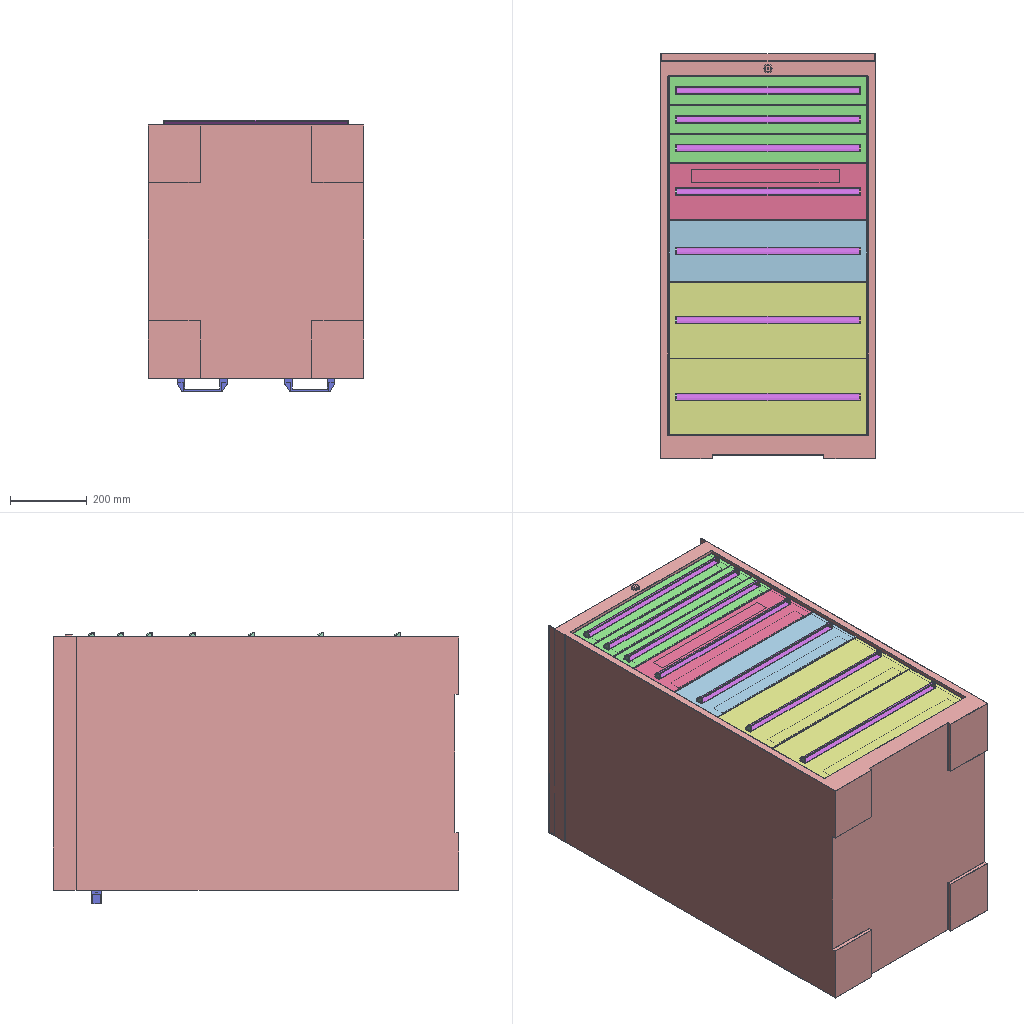Assembly | SolidWorks | 19 different items | 71 placed | box 560 x 1055 x 707 mm
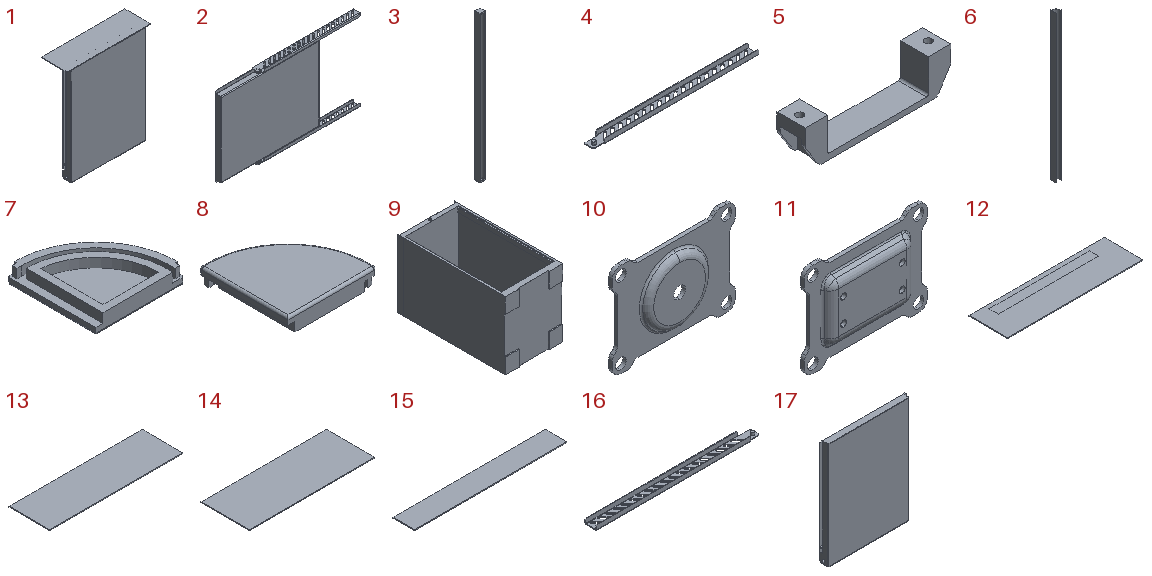Parts list (item | name | quantity | parent item | size | volume | features):
1 | (subassembly) | x1 | - | 515 x 158 x 609 mm | 1350292 mm3 | -
2 | (subassembly) | x7 | - | 859.852 x 52 x 499.996 mm | 1351190 mm3 | -
3 | (subassembly) | x7 | - | 19 x 19 x 483 mm | 27556 mm3 | -
4 | - | x7 | in 2 | 630 x 45 x 19.073 mm | 113043 mm3 | features ICE 3, SM3dBend 2, Chamfer 1, Extrusion 1, FlatPattern 1, LPattern 1, SheetMetal 1, SolidToSheetMetal 1
5 | - | x2 | - | 130 x 25 x 35 mm | 28461 mm3 | features Fillet 2, Extrusion 1, HoleWzd 1, ICE 1
6 | - | x7 | in 3 | 19 x 19 x 480 mm | 26207 mm3 | features Extrusion 1
7 | - | x7 | in 3 | 19 x 19 x 3.5 mm | 674.646 mm3 | features Extrusion 1, Fillet 1, ICE 1
8 | - | x7 | in 3 | 19 x 19 x 3.5 mm | 674.646 mm3 | features Extrusion 1, Fillet 1, ICE 1
9 | - | x1 | - | 560 x 1055 x 665 mm | 61823880 mm3 | features ICE 10, Fillet 2, Extrusion 1, HoleWzd 1
10 | - | x1 | - | 105 x 8 x 80 mm | 21623 mm3 | features ICE 3, CornerTrim 2, MirrorPattern 2, FlatPattern 1, FormToolInstance 1, HoleWzd 1, SMBaseFlange 1, SheetMetal 1
11 | - | x1 | - | 105 x 9 x 80 mm | 22120 mm3 | features ICE 3, MirrorPattern 3, CornerTrim 2, FlatPattern 1, FormToolInstance 1, HoleWzd 1, SMBaseFlange 1, SheetMetal 1
12 | - | x1 | - | 515 x 148 x 3.01 mm | 228793 mm3 | features Extrusion 1, ICE 1
13 | - | x1 | - | 515 x 158 x 3 mm | 244110 mm3 | features Extrusion 1
14 | - | x2 | - | 515 x 198 x 3 mm | 305910 mm3 | features Extrusion 1
15 | - | x3 | - | 515 x 73 x 3 mm | 112785 mm3 | features Extrusion 1
16 | - | x7 | in 2 | 630 x 45 x 19.073 mm | 113043 mm3 | features ICE 3, SM3dBend 2, Chamfer 1, Extrusion 1, FlatPattern 1, LPattern 1, SheetMetal 1, SolidToSheetMetal 1
17 | - | x7 | in 2 | 491.996 x 51.073 x 606 mm | 1106182 mm3 | features ICE 5, SM3dBend 4, Chamfer 2, Fillet 2, CosmeticWeldCutList 1, Extrusion 1, FlatPattern 1, MirrorPattern 1, SMBaseFlange 1, SheetMetal 1, SolidToSheetMetal 1
18 | angular contact ball bearing_68_skf | x1 | - | - | - | -
19 | socket head cap screw_iso | x1 | - | - | - | -
Mates (type | each side: item.copy, entity, surface, feature):
In the top assembly
Coincident | 9.1 face plane Boss-Extrude2 | 16.1 face plane Convert-Solid1
Coincident | 9.1 edge | 16.1 edge
Width | 15.1 face plane Boss-Extrude1 | 15.1 face plane Boss-Extrude1 | 17.1 face plane Sketched Bend2 | 17.1 face plane Sketched Bend1
Coincident | 17.1 face plane Boss-Extrude5 | 15.1 face plane Boss-Extrude1
DistanceDim | 17.1 face plane Boss-Extrude5 | 15.1 face plane Boss-Extrude1
DistanceDim | 9.1 face plane Cut-Extrude2 | 15.1 face plane Boss-Extrude1
LimitDistanceDim | 15.1 face plane Boss-Extrude1 | 9.1 face plane Boss-Extrude2
Coincident | 9.1 face plane Boss-Extrude2 | 16.2 face plane Convert-Solid1
Coincident | 9.1 edge | 16.2 edge
Coincident | 9.1 face plane Boss-Extrude2 | 16.3 face plane Convert-Solid1
Coincident | 9.1 edge | 16.3 edge
Coincident | 9.1 face plane Boss-Extrude2 | 16.4 face plane Convert-Solid1
Coincident | 9.1 edge | 16.4 edge
Coincident | 9.1 face plane Boss-Extrude2 | 16.5 face plane Convert-Solid1
Coincident | 9.1 edge | 16.5 edge
Coincident | 9.1 face plane Boss-Extrude2 | 16.6 face plane Convert-Solid1
Coincident | 9.1 edge | 16.6 edge
Coincident | 9.1 face plane Boss-Extrude2 | 16.7 face plane Convert-Solid1
Coincident | 9.1 edge | 16.7 edge
Coincident | 17.2 face plane Boss-Extrude5 | 15.2 face plane Boss-Extrude1
Width | 17.2 face plane Sketched Bend1 | 17.2 face plane Sketched Bend2 | 15.2 face plane Boss-Extrude1 | 15.2 face plane Boss-Extrude1
DistanceDim | 17.2 face plane Boss-Extrude5 | 15.2 face plane Boss-Extrude1
DistanceDim | 15.1 face plane Boss-Extrude1 | 15.2 face plane Boss-Extrude1
Coincident | 17.3 face plane Boss-Extrude5 | 15.3 face plane Boss-Extrude1
Width | 17.3 face plane Sketched Bend1 | 17.3 face plane Sketched Bend2 | 15.3 face plane Boss-Extrude1 | 15.3 face plane Boss-Extrude1
DistanceDim | 15.3 face plane Boss-Extrude1 | 17.3 face plane Boss-Extrude5
DistanceDim | 15.2 face plane Boss-Extrude1 | 15.3 face plane Boss-Extrude1
Coincident | 17.4 face plane Boss-Extrude5 | 12.1 face plane Boss-Extrude1
Width | 12.1 face plane Boss-Extrude1 | 12.1 face plane Boss-Extrude1 | 17.4 face plane Sketched Bend2 | 17.4 face plane Sketched Bend1
DistanceDim | 17.4 face plane Boss-Extrude5 | 12.1 face plane Boss-Extrude1
DistanceDim | 15.3 face plane Boss-Extrude1 | 12.1 face plane Boss-Extrude1
Coincident | 17.5 face plane Boss-Extrude5 | 13.1 face plane Boss-Extrude1
DistanceDim | 17.5 face plane Boss-Extrude5 | 13.1 face plane Boss-Extrude1
Width | 17.5 face plane Boss-Extrude5 | 17.5 face plane Boss-Extrude5 | 13.1 face plane Boss-Extrude1 | 13.1 face plane Boss-Extrude1
DistanceDim | 12.1 face plane Boss-Extrude1 | 13.1 face plane Boss-Extrude1
Coincident | 17.6 face plane Boss-Extrude5 | 14.1 face plane Boss-Extrude1
Width | 17.6 face plane Sketched Bend1 | 17.6 face plane Sketched Bend2 | 14.1 face plane Boss-Extrude1 | 14.1 face plane Boss-Extrude1
DistanceDim | 14.1 face plane Boss-Extrude1 | 17.6 face plane Boss-Extrude5
DistanceDim | 13.1 face plane Boss-Extrude1 | 14.1 face plane Boss-Extrude1
Coincident | 17.7 face plane Boss-Extrude5 | 14.2 face plane Boss-Extrude1
Width | 17.7 face plane Sketched Bend1 | 17.7 face plane Sketched Bend2 | 14.2 face plane Boss-Extrude1 | 14.2 face plane Boss-Extrude1
DistanceDim | 17.7 face plane Convert-Solid1 | 14.2 face plane Boss-Extrude1
DistanceDim | 14.2 face plane Boss-Extrude1 | 14.1 face plane Boss-Extrude1
LimitDistanceDim | 15.2 face plane Boss-Extrude1 | 9.1 face plane Boss-Extrude2
LimitDistanceDim | 9.1 face plane Boss-Extrude2 | 15.3 face plane Boss-Extrude1
LimitDistanceDim | 9.1 face plane Boss-Extrude2 | 12.1 face plane Boss-Extrude1
LimitDistanceDim | 13.1 face plane Boss-Extrude1 | 9.1 face plane Boss-Extrude2
LimitDistanceDim | 14.1 face plane Boss-Extrude1 | 9.1 face plane Boss-Extrude2
LimitDistanceDim | 9.1 face plane Boss-Extrude2 | 14.2 face plane Boss-Extrude1
Coincident | 15.1 face plane Boss-Extrude1 | 6.1 face plane Boss-Extrude1
Width | 8.1 face plane Boss-Extrude1 | 7.1 face plane Boss-Extrude1 | 15.1 face plane Boss-Extrude1 | 15.1 face plane Boss-Extrude1
Width | 6.1 face plane Boss-Extrude1 | 6.1 face plane Boss-Extrude1 | 15.1 face plane Boss-Extrude1 | 15.1 face plane Boss-Extrude1
Coincident | 15.2 face plane Boss-Extrude1 | 6.2 face plane Boss-Extrude1
Width | 8.2 face plane Boss-Extrude1 | 7.2 face plane Boss-Extrude1 | 15.2 face plane Boss-Extrude1 | 15.2 face plane Boss-Extrude1
Width | 6.2 face plane Boss-Extrude1 | 6.2 face plane Boss-Extrude1 | 15.2 face plane Boss-Extrude1 | 15.2 face plane Boss-Extrude1
Coincident | 15.3 face plane Boss-Extrude1 | 6.3 face plane Boss-Extrude1
Width | 8.3 face plane Boss-Extrude1 | 7.3 face plane Boss-Extrude1 | 15.3 face plane Boss-Extrude1 | 15.3 face plane Boss-Extrude1
Width | 15.3 face plane Boss-Extrude1 | 15.3 face plane Boss-Extrude1 | 6.3 face plane Boss-Extrude1 | 6.3 face plane Boss-Extrude1
Coincident | 12.1 face plane Boss-Extrude1 | 6.4 face plane Boss-Extrude1
Width | 8.4 face plane Boss-Extrude1 | 7.4 face plane Boss-Extrude1 | 12.1 face plane Boss-Extrude1 | 12.1 face plane Boss-Extrude1
Width | 6.4 face plane Boss-Extrude1 | 6.4 face plane Boss-Extrude1 | 12.1 face plane Boss-Extrude1 | 12.1 face plane Boss-Extrude1
Coincident | 13.1 face plane Boss-Extrude1 | 6.5 face plane Boss-Extrude1
Width | 8.5 face plane Boss-Extrude1 | 7.5 face plane Boss-Extrude1 | 13.1 face plane Boss-Extrude1 | 13.1 face plane Boss-Extrude1
Width | 6.5 face plane Boss-Extrude1 | 6.5 face plane Boss-Extrude1 | 13.1 face plane Boss-Extrude1 | 13.1 face plane Boss-Extrude1
Coincident | 14.1 face plane Boss-Extrude1 | 6.6 face plane Boss-Extrude1
Width | 6.6 face plane Boss-Extrude1 | 6.6 face plane Boss-Extrude1 | 14.1 face plane Boss-Extrude1 | 14.1 face plane Boss-Extrude1
Width | 14.1 face plane Boss-Extrude1 | 14.1 face plane Boss-Extrude1 | 8.6 face plane Boss-Extrude1 | 7.6 face plane Boss-Extrude1
Coincident | 14.2 face plane Boss-Extrude1 | 6.7 face plane Boss-Extrude1
Width | 8.7 face plane Boss-Extrude1 | 7.7 face plane Boss-Extrude1 | 14.2 face plane Boss-Extrude1 | 14.2 face plane Boss-Extrude1
Width | 6.7 face plane Boss-Extrude1 | 6.7 face plane Boss-Extrude1 | 14.2 face plane Boss-Extrude1 | 14.2 face plane Boss-Extrude1
Coincident | 9.1 face plane Boss-Extrude1 | 5.1 face plane Boss-Extrude1
Coincident | 9.1 face plane Boss-Extrude1 | 5.2 face plane Boss-Extrude1
Coincident | 5.2 face plane Boss-Extrude1 | 5.1 face plane Boss-Extrude1
DistanceDim | 5.1 face plane Boss-Extrude1 | 9.1 face plane Boss-Extrude1 | 2 times
DistanceDim | 5.2 face plane Boss-Extrude1 | 9.1 face plane Boss-Extrude1
In subassembly 3
Coincident | 6.8 face plane Boss-Extrude1 | 8.8 face plane Boss-Extrude1 | 2 times
Coincident | 6.8 vertex | 8.8 face plane Boss-Extrude1
Coincident | 6.8 face plane Boss-Extrude1 | 7.8 face plane Boss-Extrude1 | 3 times
In subassembly 2
Parallel | 4.1 face plane Sketched Bend1 | 17.8 face plane Convert-Solid1
Parallel | 17.8 face plane Sketched Bend4 | 16.8 face plane Sketched Bend2
Coincident | 4.1 face plane Convert-Solid1 | 16.8 face plane Convert-Solid1